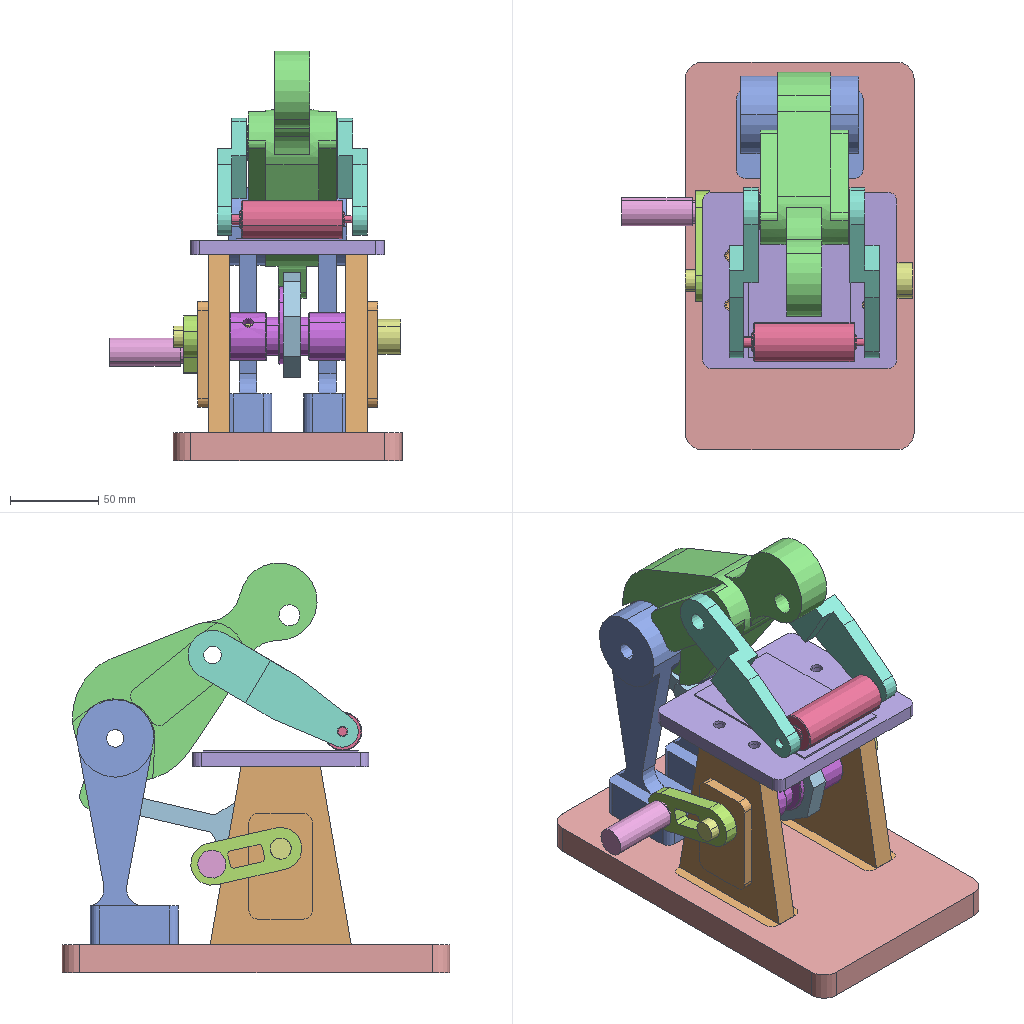Assembly | SolidWorks | 12 different items | 15 placed | box 166 x 220 x 232 mm
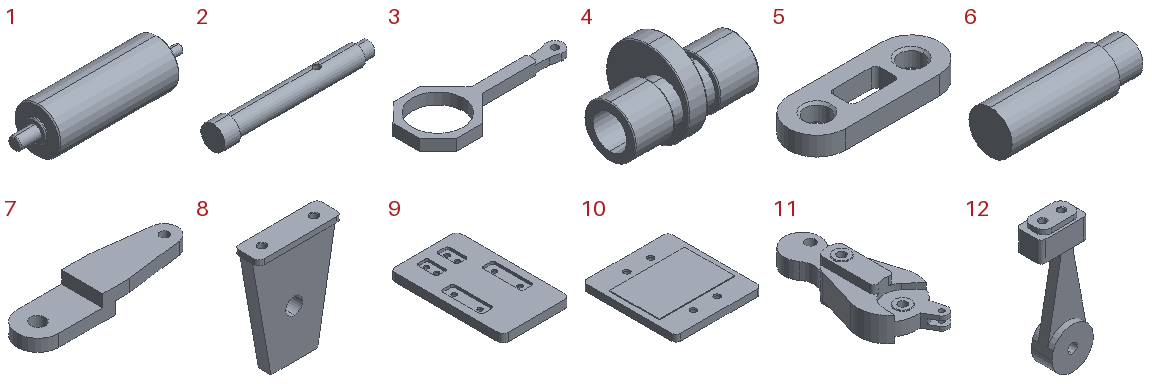Parts list (item | quantity | size | volume | features):
1 | x1 | 79.6 x 22 x 22 mm | 22421 mm3 | features Chamfer 1, Revolution 1
2 | x1 | 129 x 20 x 20 mm | 26391 mm3 | features 3DProfileFeature 1, HoleWzd 1, Revolution 1
3 | x1 | 139.5 x 56 x 10 mm | 17824 mm3 | features ICE 2, Extrusion 1
4 | x1 | 66 x 44 x 44 mm | 29541 mm3 | features ICE 3, Fillet 1, Revolution 1
5 | x1 | 64 x 24 x 8 mm | 8361 mm3 | features MirrorPattern 2, 3DProfileFeature 1, Extrusion 1, HoleWzd 1
6 | x1 | 50 x 16 x 16 mm | 9370 mm3 | features Revolution 1
7 | x2 | 108.5 x 28 x 16.6 mm | 22997 mm3 | features Extrusion 1, ICE 1
8 | x2 | 80 x 24 x 106 mm | 92527 mm3 | features ICE 3, 3DProfileFeature 2, HoleWzd 2, Extrusion 1
9 | x1 | 130 x 220 x 16 mm | 415367 mm3 | features ICE 3, Extrusion 1
10 | x1 | 100 x 110 x 9 mm | 89910 mm3 | features ICE 3, Extrusion 1
11 | x1 | 72 x 180.817 x 52 mm | 220278 mm3 | features ICE 9, Chamfer 2, MirrorPattern 2, Extrusion 1
12 | x2 | 57.8 x 27 x 144 mm | 81593 mm3 | features ICE 3, 3DProfileFeature 1, Extrusion 1, HoleWzd 1
Mates (type | each side: item.copy, entity, surface, feature):
Concentric | 7.1 face cylinder Boss-Extrude2 | 11.1 face cylinder Cut-Extrude3
Coincident | 7.1 face plane Boss-Extrude2 | 11.1 face plane Boss-Extrude4
Concentric | 11.1 face cylinder Cut-Extrude3 | 7.2 face cylinder Boss-Extrude2
Coincident | 11.1 face plane Mirror2 | 7.2 face plane Boss-Extrude2
Concentric | 12.1 face cylinder Boss-Extrude4 | 11.1 face cylinder Mirror1
Coincident | 12.1 face plane Boss-Extrude4 | 11.1 face plane Mirror2
Concentric | 9.1 face cylinder Cut-Extrude1 | 12.1 face cylinder Boss-Extrude1
Parallel | 9.1 face plane Cut-Extrude1 | 12.1 face plane Boss-Extrude1
Coincident | 9.1 face plane Cut-Extrude1 | 12.1 face plane Boss-Extrude2
Concentric | 7.1 face cylinder Boss-Extrude4 | 7.2 face cylinder Boss-Extrude4
Coincident | 9.1 face plane Cut-Extrude1 | 8.1 face plane Boss-Extrude1 | 2 times
Concentric | 9.1 face cylinder Cut-Extrude1 | 8.1 face cylinder Boss-Extrude1
Concentric | 8.1 face cylinder M6 Tapped Hole1 | 10.1 edge
Parallel | 8.1 face plane Boss-Extrude2 | 10.1 face plane Boss-Extrude1
Coincident | 8.1 face plane Boss-Extrude2 | 10.1 face plane Boss-Extrude1
Concentric | 11.1 face cylinder Cut-Extrude5 | 3.1 face cylinder Cut-Extrude1
Coincident | 11.1 face plane Cut-Extrude4 | 3.1 face plane Boss-Extrude2
Concentric | 7.1 face cylinder Boss-Extrude4 | 1.1 face cylinder Revolve1
DistanceDim | 1.1 face plane Revolve1 | 7.2 face plane Boss-Extrude4
Tangent | 10.1 face plane Boss-Extrude2 | 1.1 face cylinder Revolve1
Coincident | 5.1 face plane Boss-Extrude1 | 8.1 face plane Boss-Extrude3
Concentric | 5.1 face cylinder Mirror2 | 6.1 face cylinder Revolve1
Coincident | 5.1 face plane Boss-Extrude1 | 6.1 face plane Revolve1
Concentric | 8.1 face cylinder Cut-Extrude1 | 2.1 face cylinder Revolve1
Coincident | 8.2 face plane Boss-Extrude3 | 2.1 face plane Revolve1
Concentric | 5.1 face cylinder M12 Tapped Hole1 | 2.1 face cylinder Revolve1
Concentric | 2.1 face cylinder Revolve1 | 4.1 face cylinder Revolve1
Concentric | 2.1 face cylinder M6 Tapped Hole2 | 4.1 face cylinder Cut-Extrude2
Concentric | 3.1 face cylinder Boss-Extrude1 | 4.1 face cylinder Boss-Extrude1
Lock | 5.1 select_type:0 | 2.1 select_type:0